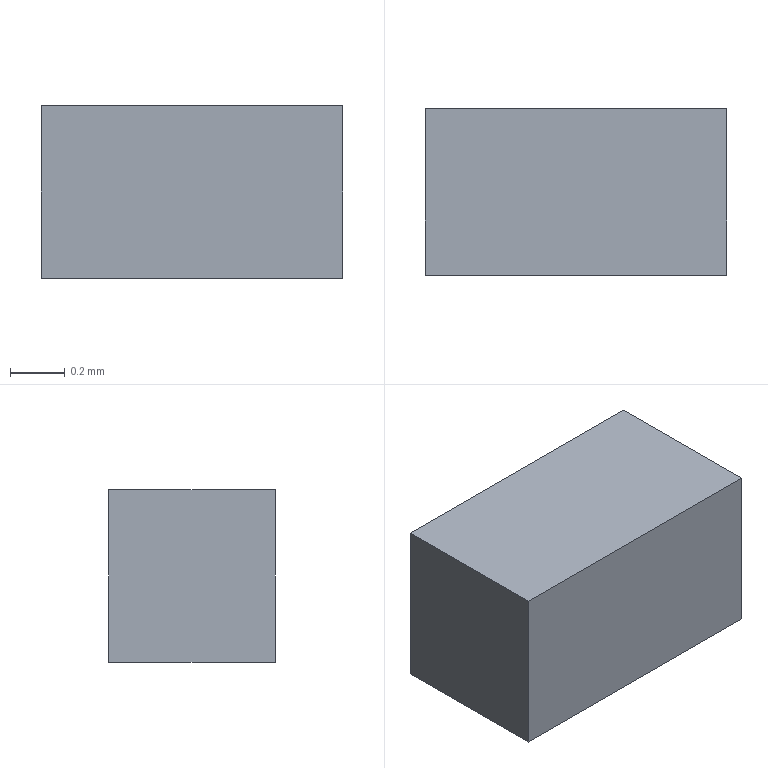Part | Creo | 1 solid | 6 faces | box 1.107 x 0.6124 x 0.6325 mm | volume 0.4288 mm3 | plane 6
STEP:
#1=CARTESIAN_POINT('',(0.,0.,0.));
#2=DIRECTION('',(0.,0.,1.));
#3=DIRECTION('',(1.,0.,0.));
#4=AXIS2_PLACEMENT_3D('',#1,#2,#3);
#5=CARTESIAN_POINT('',(-0.5819,-0.3374,0.));
#6=VERTEX_POINT('',#5);
#7=CARTESIAN_POINT('',(0.525,-0.3374,0.));
#8=VERTEX_POINT('',#7);
#9=CARTESIAN_POINT('',(-0.5819,-0.3374,0.));
#10=DIRECTION('',(1.,0.,0.));
#11=VECTOR('',#10,1.107);
#12=LINE('',#9,#11);
#13=EDGE_CURVE('',#6,#8,#12,.T.);
#14=ORIENTED_EDGE('',*,*,#13,.T.);
#15=CARTESIAN_POINT('',(0.525,0.275,0.));
#16=VERTEX_POINT('',#15);
#17=CARTESIAN_POINT('',(0.525,-0.3374,0.));
#18=DIRECTION('',(0.,1.,0.));
#19=VECTOR('',#18,0.6124);
#20=LINE('',#17,#19);
#21=EDGE_CURVE('',#8,#16,#20,.T.);
#22=ORIENTED_EDGE('',*,*,#21,.T.);
#23=CARTESIAN_POINT('',(-0.5819,0.275,0.));
#24=VERTEX_POINT('',#23);
#25=CARTESIAN_POINT('',(0.525,0.275,0.));
#26=DIRECTION('',(-1.,0.,0.));
#27=VECTOR('',#26,1.107);
#28=LINE('',#25,#27);
#29=EDGE_CURVE('',#16,#24,#28,.T.);
#30=ORIENTED_EDGE('',*,*,#29,.T.);
#31=CARTESIAN_POINT('',(-0.5819,0.275,0.));
#32=DIRECTION('',(0.,-1.,0.));
#33=VECTOR('',#32,0.6124);
#34=LINE('',#31,#33);
#35=EDGE_CURVE('',#24,#6,#34,.T.);
#36=ORIENTED_EDGE('',*,*,#35,.T.);
#37=EDGE_LOOP('',(#14,#22,#30,#36));
#38=FACE_OUTER_BOUND('',#37,.F.);
#39=CARTESIAN_POINT('',(0.,0.,0.));
#40=DIRECTION('',(0.,0.,1.));
#41=DIRECTION('',(1.,0.,0.));
#42=AXIS2_PLACEMENT_3D('',#39,#40,#41);
#43=PLANE('',#42);
#44=ADVANCED_FACE('',(#38),#43,.F.);
#45=ORIENTED_EDGE('',*,*,#13,.F.);
#46=CARTESIAN_POINT('',(-0.5819,-0.3374,0.6325));
#47=VERTEX_POINT('',#46);
#48=CARTESIAN_POINT('',(-0.5819,-0.3374,0.));
#49=DIRECTION('',(0.,0.,1.));
#50=VECTOR('',#49,0.6325);
#51=LINE('',#48,#50);
#52=EDGE_CURVE('',#6,#47,#51,.T.);
#53=ORIENTED_EDGE('',*,*,#52,.T.);
#54=CARTESIAN_POINT('',(0.525,-0.3374,0.6325));
#55=VERTEX_POINT('',#54);
#56=CARTESIAN_POINT('',(-0.5819,-0.3374,0.6325));
#57=DIRECTION('',(1.,0.,0.));
#58=VECTOR('',#57,1.107);
#59=LINE('',#56,#58);
#60=EDGE_CURVE('',#47,#55,#59,.T.);
#61=ORIENTED_EDGE('',*,*,#60,.T.);
#62=CARTESIAN_POINT('',(0.525,-0.3374,0.));
#63=DIRECTION('',(0.,0.,1.));
#64=VECTOR('',#63,0.6325);
#65=LINE('',#62,#64);
#66=EDGE_CURVE('',#8,#55,#65,.T.);
#67=ORIENTED_EDGE('',*,*,#66,.F.);
#68=EDGE_LOOP('',(#45,#53,#61,#67));
#69=FACE_OUTER_BOUND('',#68,.F.);
#70=CARTESIAN_POINT('',(-0.5819,-0.3374,0.));
#71=DIRECTION('',(0.,-1.,0.));
#72=DIRECTION('',(1.,0.,0.));
#73=AXIS2_PLACEMENT_3D('',#70,#71,#72);
#74=PLANE('',#73);
#75=ADVANCED_FACE('',(#69),#74,.T.);
#76=ORIENTED_EDGE('',*,*,#35,.F.);
#77=CARTESIAN_POINT('',(-0.5819,0.275,0.6325));
#78=VERTEX_POINT('',#77);
#79=CARTESIAN_POINT('',(-0.5819,0.275,0.));
#80=DIRECTION('',(0.,0.,1.));
#81=VECTOR('',#80,0.6325);
#82=LINE('',#79,#81);
#83=EDGE_CURVE('',#24,#78,#82,.T.);
#84=ORIENTED_EDGE('',*,*,#83,.T.);
#85=CARTESIAN_POINT('',(-0.5819,0.275,0.6325));
#86=DIRECTION('',(0.,-1.,0.));
#87=VECTOR('',#86,0.6124);
#88=LINE('',#85,#87);
#89=EDGE_CURVE('',#78,#47,#88,.T.);
#90=ORIENTED_EDGE('',*,*,#89,.T.);
#91=ORIENTED_EDGE('',*,*,#52,.F.);
#92=EDGE_LOOP('',(#76,#84,#90,#91));
#93=FACE_OUTER_BOUND('',#92,.F.);
#94=CARTESIAN_POINT('',(-0.5819,0.275,0.));
#95=DIRECTION('',(-1.,0.,0.));
#96=DIRECTION('',(0.,-1.,0.));
#97=AXIS2_PLACEMENT_3D('',#94,#95,#96);
#98=PLANE('',#97);
#99=ADVANCED_FACE('',(#93),#98,.T.);
#100=ORIENTED_EDGE('',*,*,#29,.F.);
#101=CARTESIAN_POINT('',(0.525,0.275,0.6325));
#102=VERTEX_POINT('',#101);
#103=CARTESIAN_POINT('',(0.525,0.275,0.));
#104=DIRECTION('',(0.,0.,1.));
#105=VECTOR('',#104,0.6325);
#106=LINE('',#103,#105);
#107=EDGE_CURVE('',#16,#102,#106,.T.);
#108=ORIENTED_EDGE('',*,*,#107,.T.);
#109=CARTESIAN_POINT('',(0.525,0.275,0.6325));
#110=DIRECTION('',(-1.,0.,0.));
#111=VECTOR('',#110,1.107);
#112=LINE('',#109,#111);
#113=EDGE_CURVE('',#102,#78,#112,.T.);
#114=ORIENTED_EDGE('',*,*,#113,.T.);
#115=ORIENTED_EDGE('',*,*,#83,.F.);
#116=EDGE_LOOP('',(#100,#108,#114,#115));
#117=FACE_OUTER_BOUND('',#116,.F.);
#118=CARTESIAN_POINT('',(0.525,0.275,0.));
#119=DIRECTION('',(0.,1.,0.));
#120=DIRECTION('',(-1.,0.,0.));
#121=AXIS2_PLACEMENT_3D('',#118,#119,#120);
#122=PLANE('',#121);
#123=ADVANCED_FACE('',(#117),#122,.T.);
#124=ORIENTED_EDGE('',*,*,#21,.F.);
#125=ORIENTED_EDGE('',*,*,#66,.T.);
#126=CARTESIAN_POINT('',(0.525,-0.3374,0.6325));
#127=DIRECTION('',(0.,1.,0.));
#128=VECTOR('',#127,0.6124);
#129=LINE('',#126,#128);
#130=EDGE_CURVE('',#55,#102,#129,.T.);
#131=ORIENTED_EDGE('',*,*,#130,.T.);
#132=ORIENTED_EDGE('',*,*,#107,.F.);
#133=EDGE_LOOP('',(#124,#125,#131,#132));
#134=FACE_OUTER_BOUND('',#133,.F.);
#135=CARTESIAN_POINT('',(0.525,-0.3374,0.));
#136=DIRECTION('',(1.,0.,0.));
#137=DIRECTION('',(0.,1.,0.));
#138=AXIS2_PLACEMENT_3D('',#135,#136,#137);
#139=PLANE('',#138);
#140=ADVANCED_FACE('',(#134),#139,.T.);
#141=ORIENTED_EDGE('',*,*,#60,.F.);
#142=ORIENTED_EDGE('',*,*,#89,.F.);
#143=ORIENTED_EDGE('',*,*,#113,.F.);
#144=ORIENTED_EDGE('',*,*,#130,.F.);
#145=EDGE_LOOP('',(#141,#142,#143,#144));
#146=FACE_OUTER_BOUND('',#145,.F.);
#147=CARTESIAN_POINT('',(0.,0.,0.6325));
#148=DIRECTION('',(0.,0.,1.));
#149=DIRECTION('',(1.,0.,0.));
#150=AXIS2_PLACEMENT_3D('',#147,#148,#149);
#151=PLANE('',#150);
#152=ADVANCED_FACE('',(#146),#151,.T.);
#153=CLOSED_SHELL('',(#44,#75,#99,#123,#140,#152));
#154=MANIFOLD_SOLID_BREP('',#153);
#155=(LENGTH_UNIT()NAMED_UNIT(*)SI_UNIT(.MILLI.,.METRE.));
#156=UNCERTAINTY_MEASURE_WITH_UNIT(LENGTH_MEASURE(0.0001414),#155,'','');
#157=(NAMED_UNIT(*)PLANE_ANGLE_UNIT()SI_UNIT($,.RADIAN.));
#158=PLANE_ANGLE_MEASURE_WITH_UNIT(PLANE_ANGLE_MEASURE(0.01745),#157);
#159=(CONVERSION_BASED_UNIT('DEGREE',#158)NAMED_UNIT(*)PLANE_ANGLE_UNIT());
#160=(NAMED_UNIT(*)SI_UNIT($,.STERADIAN.)SOLID_ANGLE_UNIT());
#161=(GEOMETRIC_REPRESENTATION_CONTEXT(3)GLOBAL_UNCERTAINTY_ASSIGNED_CONTEXT((#156))GLOBAL_UNIT_ASSIGNED_CONTEXT((#155,#159,#160))REPRESENTATION_CONTEXT('',''));
#162=ADVANCED_BREP_SHAPE_REPRESENTATION('',(#4,#154),#161);